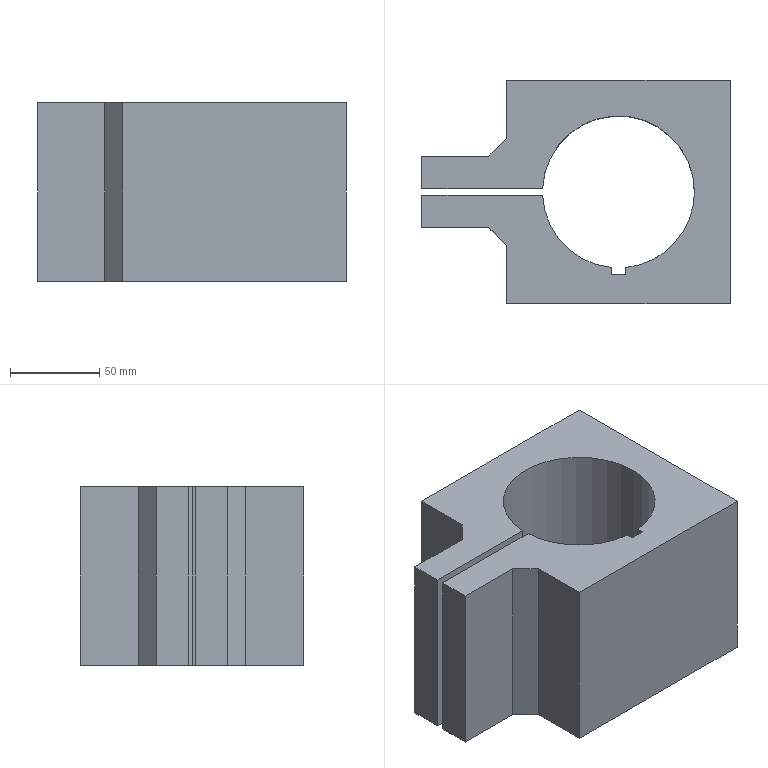Part | STEP file | csb-00001 | 1 solid | 21 faces | box 172.5 x 125 x 100 mm | volume 1165193 mm3 | plane 18 | cylinder 3 | commonest cylinder face diameters 85 x3
STEP:
#1=CARTESIAN_POINT('',(-42.453,2.,-100.));
#2=VERTEX_POINT('',#1);
#3=CARTESIAN_POINT('',(42.5,0.,-100.));
#4=VERTEX_POINT('',#3);
#5=CARTESIAN_POINT('',(0.,0.,-100.));
#6=DIRECTION('',(0.,0.,-1.));
#7=DIRECTION('',(1.,0.,0.));
#8=AXIS2_PLACEMENT_3D('',#5,#6,#7);
#9=CIRCLE('',#8,42.5);
#10=EDGE_CURVE('',#2,#4,#9,.T.);
#11=ORIENTED_EDGE('',*,*,#10,.T.);
#12=CARTESIAN_POINT('',(42.5,0.,0.));
#13=VERTEX_POINT('',#12);
#14=CARTESIAN_POINT('',(42.5,0.,-100.));
#15=DIRECTION('',(0.,0.,1.));
#16=VECTOR('',#15,1000.);
#17=LINE('',#14,#16);
#18=EDGE_CURVE('',#4,#13,#17,.T.);
#19=ORIENTED_EDGE('',*,*,#18,.T.);
#20=CARTESIAN_POINT('',(-42.453,2.,0.));
#21=VERTEX_POINT('',#20);
#22=CARTESIAN_POINT('',(0.,0.,0.));
#23=DIRECTION('',(0.,0.,-1.));
#24=DIRECTION('',(1.,0.,0.));
#25=AXIS2_PLACEMENT_3D('',#22,#23,#24);
#26=CIRCLE('',#25,42.5);
#27=EDGE_CURVE('',#21,#13,#26,.T.);
#28=ORIENTED_EDGE('',*,*,#27,.F.);
#29=CARTESIAN_POINT('',(-42.453,2.,-100.));
#30=DIRECTION('',(0.,0.,1.));
#31=VECTOR('',#30,1000.);
#32=LINE('',#29,#31);
#33=EDGE_CURVE('',#2,#21,#32,.T.);
#34=ORIENTED_EDGE('',*,*,#33,.F.);
#35=EDGE_LOOP('',(#11,#19,#28,#34));
#36=FACE_OUTER_BOUND('',#35,.T.);
#37=CARTESIAN_POINT('',(0.,0.,-100.));
#38=DIRECTION('',(0.,0.,1.));
#39=DIRECTION('',(1.,0.,0.));
#40=AXIS2_PLACEMENT_3D('',#37,#38,#39);
#41=CYLINDRICAL_SURFACE('',#40,42.5);
#42=ADVANCED_FACE('',(#36),#41,.F.);
#43=CARTESIAN_POINT('',(62.5,-62.5,0.));
#44=VERTEX_POINT('',#43);
#45=CARTESIAN_POINT('',(62.5,62.5,0.));
#46=VERTEX_POINT('',#45);
#47=CARTESIAN_POINT('',(62.5,-62.5,0.));
#48=DIRECTION('',(0.,1.,0.));
#49=VECTOR('',#48,1000.);
#50=LINE('',#47,#49);
#51=EDGE_CURVE('',#44,#46,#50,.T.);
#52=ORIENTED_EDGE('',*,*,#51,.F.);
#53=CARTESIAN_POINT('',(62.5,-62.5,-100.));
#54=VERTEX_POINT('',#53);
#55=CARTESIAN_POINT('',(62.5,-62.5,-100.));
#56=DIRECTION('',(0.,0.,1.));
#57=VECTOR('',#56,1000.);
#58=LINE('',#55,#57);
#59=EDGE_CURVE('',#54,#44,#58,.T.);
#60=ORIENTED_EDGE('',*,*,#59,.F.);
#61=CARTESIAN_POINT('',(62.5,62.5,-100.));
#62=VERTEX_POINT('',#61);
#63=CARTESIAN_POINT('',(62.5,-62.5,-100.));
#64=DIRECTION('',(0.,1.,0.));
#65=VECTOR('',#64,1000.);
#66=LINE('',#63,#65);
#67=EDGE_CURVE('',#54,#62,#66,.T.);
#68=ORIENTED_EDGE('',*,*,#67,.T.);
#69=CARTESIAN_POINT('',(62.5,62.5,-100.));
#70=DIRECTION('',(0.,0.,1.));
#71=VECTOR('',#70,1000.);
#72=LINE('',#69,#71);
#73=EDGE_CURVE('',#62,#46,#72,.T.);
#74=ORIENTED_EDGE('',*,*,#73,.T.);
#75=EDGE_LOOP('',(#52,#60,#68,#74));
#76=FACE_OUTER_BOUND('',#75,.T.);
#77=CARTESIAN_POINT('',(62.5,-62.5,-100.));
#78=DIRECTION('',(1.,0.,0.));
#79=DIRECTION('',(0.,0.,-1.));
#80=AXIS2_PLACEMENT_3D('',#77,#78,#79);
#81=PLANE('',#80);
#82=ADVANCED_FACE('',(#76),#81,.T.);
#83=CARTESIAN_POINT('',(-62.5,-62.5,0.));
#84=VERTEX_POINT('',#83);
#85=CARTESIAN_POINT('',(-62.5,-62.5,0.));
#86=DIRECTION('',(1.,0.,0.));
#87=VECTOR('',#86,1000.);
#88=LINE('',#85,#87);
#89=EDGE_CURVE('',#84,#44,#88,.T.);
#90=ORIENTED_EDGE('',*,*,#89,.F.);
#91=CARTESIAN_POINT('',(-62.5,-62.5,-100.));
#92=VERTEX_POINT('',#91);
#93=CARTESIAN_POINT('',(-62.5,-62.5,-100.));
#94=DIRECTION('',(0.,0.,1.));
#95=VECTOR('',#94,1000.);
#96=LINE('',#93,#95);
#97=EDGE_CURVE('',#92,#84,#96,.T.);
#98=ORIENTED_EDGE('',*,*,#97,.F.);
#99=CARTESIAN_POINT('',(-62.5,-62.5,-100.));
#100=DIRECTION('',(1.,0.,0.));
#101=VECTOR('',#100,1000.);
#102=LINE('',#99,#101);
#103=EDGE_CURVE('',#92,#54,#102,.T.);
#104=ORIENTED_EDGE('',*,*,#103,.T.);
#105=ORIENTED_EDGE('',*,*,#59,.T.);
#106=EDGE_LOOP('',(#90,#98,#104,#105));
#107=FACE_OUTER_BOUND('',#106,.T.);
#108=CARTESIAN_POINT('',(-62.5,-62.5,-100.));
#109=DIRECTION('',(0.,-1.,0.));
#110=DIRECTION('',(0.,0.,-1.));
#111=AXIS2_PLACEMENT_3D('',#108,#109,#110);
#112=PLANE('',#111);
#113=ADVANCED_FACE('',(#107),#112,.T.);
#114=CARTESIAN_POINT('',(-62.5,-30.,0.));
#115=VERTEX_POINT('',#114);
#116=CARTESIAN_POINT('',(-62.5,-62.5,0.));
#117=DIRECTION('',(0.,-1.,0.));
#118=VECTOR('',#117,1000.);
#119=LINE('',#116,#118);
#120=EDGE_CURVE('',#115,#84,#119,.T.);
#121=ORIENTED_EDGE('',*,*,#120,.F.);
#122=CARTESIAN_POINT('',(-62.5,-30.,-100.));
#123=VERTEX_POINT('',#122);
#124=CARTESIAN_POINT('',(-62.5,-30.,-100.));
#125=DIRECTION('',(0.,0.,1.));
#126=VECTOR('',#125,1000.);
#127=LINE('',#124,#126);
#128=EDGE_CURVE('',#123,#115,#127,.T.);
#129=ORIENTED_EDGE('',*,*,#128,.F.);
#130=CARTESIAN_POINT('',(-62.5,-62.5,-100.));
#131=DIRECTION('',(0.,-1.,0.));
#132=VECTOR('',#131,1000.);
#133=LINE('',#130,#132);
#134=EDGE_CURVE('',#123,#92,#133,.T.);
#135=ORIENTED_EDGE('',*,*,#134,.T.);
#136=ORIENTED_EDGE('',*,*,#97,.T.);
#137=EDGE_LOOP('',(#121,#129,#135,#136));
#138=FACE_OUTER_BOUND('',#137,.T.);
#139=CARTESIAN_POINT('',(-62.5,-62.5,-100.));
#140=DIRECTION('',(-1.,0.,0.));
#141=DIRECTION('',(0.,0.,1.));
#142=AXIS2_PLACEMENT_3D('',#139,#140,#141);
#143=PLANE('',#142);
#144=ADVANCED_FACE('',(#138),#143,.T.);
#145=CARTESIAN_POINT('',(-72.5,-20.,0.));
#146=VERTEX_POINT('',#145);
#147=CARTESIAN_POINT('',(-72.5,-20.,0.));
#148=DIRECTION('',(0.7071,-0.7071,0.));
#149=VECTOR('',#148,1000.);
#150=LINE('',#147,#149);
#151=EDGE_CURVE('',#146,#115,#150,.T.);
#152=ORIENTED_EDGE('',*,*,#151,.F.);
#153=CARTESIAN_POINT('',(-72.5,-20.,-100.));
#154=VERTEX_POINT('',#153);
#155=CARTESIAN_POINT('',(-72.5,-20.,-100.));
#156=DIRECTION('',(0.,0.,1.));
#157=VECTOR('',#156,1000.);
#158=LINE('',#155,#157);
#159=EDGE_CURVE('',#154,#146,#158,.T.);
#160=ORIENTED_EDGE('',*,*,#159,.F.);
#161=CARTESIAN_POINT('',(-72.5,-20.,-100.));
#162=DIRECTION('',(0.7071,-0.7071,0.));
#163=VECTOR('',#162,1000.);
#164=LINE('',#161,#163);
#165=EDGE_CURVE('',#154,#123,#164,.T.);
#166=ORIENTED_EDGE('',*,*,#165,.T.);
#167=ORIENTED_EDGE('',*,*,#128,.T.);
#168=EDGE_LOOP('',(#152,#160,#166,#167));
#169=FACE_OUTER_BOUND('',#168,.T.);
#170=CARTESIAN_POINT('',(-72.5,-20.,-100.));
#171=DIRECTION('',(-0.7071,-0.7071,0.));
#172=DIRECTION('',(0.7071,-0.7071,0.));
#173=AXIS2_PLACEMENT_3D('',#170,#171,#172);
#174=PLANE('',#173);
#175=ADVANCED_FACE('',(#169),#174,.T.);
#176=CARTESIAN_POINT('',(-110.,-20.,0.));
#177=VERTEX_POINT('',#176);
#178=CARTESIAN_POINT('',(-110.,-20.,0.));
#179=DIRECTION('',(1.,0.,0.));
#180=VECTOR('',#179,1000.);
#181=LINE('',#178,#180);
#182=EDGE_CURVE('',#177,#146,#181,.T.);
#183=ORIENTED_EDGE('',*,*,#182,.F.);
#184=CARTESIAN_POINT('',(-110.,-20.,-100.));
#185=VERTEX_POINT('',#184);
#186=CARTESIAN_POINT('',(-110.,-20.,-100.));
#187=DIRECTION('',(0.,0.,1.));
#188=VECTOR('',#187,1000.);
#189=LINE('',#186,#188);
#190=EDGE_CURVE('',#185,#177,#189,.T.);
#191=ORIENTED_EDGE('',*,*,#190,.F.);
#192=CARTESIAN_POINT('',(-110.,-20.,-100.));
#193=DIRECTION('',(1.,0.,0.));
#194=VECTOR('',#193,1000.);
#195=LINE('',#192,#194);
#196=EDGE_CURVE('',#185,#154,#195,.T.);
#197=ORIENTED_EDGE('',*,*,#196,.T.);
#198=ORIENTED_EDGE('',*,*,#159,.T.);
#199=EDGE_LOOP('',(#183,#191,#197,#198));
#200=FACE_OUTER_BOUND('',#199,.T.);
#201=CARTESIAN_POINT('',(-110.,-20.,-100.));
#202=DIRECTION('',(0.,-1.,0.));
#203=DIRECTION('',(1.,0.,0.));
#204=AXIS2_PLACEMENT_3D('',#201,#202,#203);
#205=PLANE('',#204);
#206=ADVANCED_FACE('',(#200),#205,.T.);
#207=CARTESIAN_POINT('',(-110.,-2.,0.));
#208=VERTEX_POINT('',#207);
#209=CARTESIAN_POINT('',(-110.,-20.,0.));
#210=DIRECTION('',(0.,-1.,0.));
#211=VECTOR('',#210,1000.);
#212=LINE('',#209,#211);
#213=EDGE_CURVE('',#208,#177,#212,.T.);
#214=ORIENTED_EDGE('',*,*,#213,.F.);
#215=CARTESIAN_POINT('',(-110.,-2.,-100.));
#216=VERTEX_POINT('',#215);
#217=CARTESIAN_POINT('',(-110.,-2.,-100.));
#218=DIRECTION('',(0.,0.,1.));
#219=VECTOR('',#218,1000.);
#220=LINE('',#217,#219);
#221=EDGE_CURVE('',#216,#208,#220,.T.);
#222=ORIENTED_EDGE('',*,*,#221,.F.);
#223=CARTESIAN_POINT('',(-110.,-20.,-100.));
#224=DIRECTION('',(0.,-1.,0.));
#225=VECTOR('',#224,1000.);
#226=LINE('',#223,#225);
#227=EDGE_CURVE('',#216,#185,#226,.T.);
#228=ORIENTED_EDGE('',*,*,#227,.T.);
#229=ORIENTED_EDGE('',*,*,#190,.T.);
#230=EDGE_LOOP('',(#214,#222,#228,#229));
#231=FACE_OUTER_BOUND('',#230,.T.);
#232=CARTESIAN_POINT('',(-110.,-20.,-100.));
#233=DIRECTION('',(-1.,0.,0.));
#234=DIRECTION('',(0.,-1.,0.));
#235=AXIS2_PLACEMENT_3D('',#232,#233,#234);
#236=PLANE('',#235);
#237=ADVANCED_FACE('',(#231),#236,.T.);
#238=CARTESIAN_POINT('',(-42.453,-2.,0.));
#239=VERTEX_POINT('',#238);
#240=CARTESIAN_POINT('',(-110.,-2.,0.));
#241=DIRECTION('',(-1.,0.,0.));
#242=VECTOR('',#241,1000.);
#243=LINE('',#240,#242);
#244=EDGE_CURVE('',#239,#208,#243,.T.);
#245=ORIENTED_EDGE('',*,*,#244,.F.);
#246=CARTESIAN_POINT('',(-42.453,-2.,-100.));
#247=VERTEX_POINT('',#246);
#248=CARTESIAN_POINT('',(-42.453,-2.,-100.));
#249=DIRECTION('',(0.,0.,1.));
#250=VECTOR('',#249,1000.);
#251=LINE('',#248,#250);
#252=EDGE_CURVE('',#247,#239,#251,.T.);
#253=ORIENTED_EDGE('',*,*,#252,.F.);
#254=CARTESIAN_POINT('',(-110.,-2.,-100.));
#255=DIRECTION('',(-1.,0.,0.));
#256=VECTOR('',#255,1000.);
#257=LINE('',#254,#256);
#258=EDGE_CURVE('',#247,#216,#257,.T.);
#259=ORIENTED_EDGE('',*,*,#258,.T.);
#260=ORIENTED_EDGE('',*,*,#221,.T.);
#261=EDGE_LOOP('',(#245,#253,#259,#260));
#262=FACE_OUTER_BOUND('',#261,.T.);
#263=CARTESIAN_POINT('',(-110.,-2.,-100.));
#264=DIRECTION('',(0.,1.,0.));
#265=DIRECTION('',(0.,0.,1.));
#266=AXIS2_PLACEMENT_3D('',#263,#264,#265);
#267=PLANE('',#266);
#268=ADVANCED_FACE('',(#262),#267,.T.);
#269=CARTESIAN_POINT('',(-4.,-42.311,0.));
#270=VERTEX_POINT('',#269);
#271=CARTESIAN_POINT('',(0.,0.,0.));
#272=DIRECTION('',(0.,0.,-1.));
#273=DIRECTION('',(1.,0.,0.));
#274=AXIS2_PLACEMENT_3D('',#271,#272,#273);
#275=CIRCLE('',#274,42.5);
#276=EDGE_CURVE('',#270,#239,#275,.T.);
#277=ORIENTED_EDGE('',*,*,#276,.F.);
#278=CARTESIAN_POINT('',(-4.,-42.311,-100.));
#279=VERTEX_POINT('',#278);
#280=CARTESIAN_POINT('',(-4.,-42.311,-100.));
#281=DIRECTION('',(0.,0.,1.));
#282=VECTOR('',#281,1000.);
#283=LINE('',#280,#282);
#284=EDGE_CURVE('',#279,#270,#283,.T.);
#285=ORIENTED_EDGE('',*,*,#284,.F.);
#286=CARTESIAN_POINT('',(0.,0.,-100.));
#287=DIRECTION('',(0.,0.,-1.));
#288=DIRECTION('',(1.,0.,0.));
#289=AXIS2_PLACEMENT_3D('',#286,#287,#288);
#290=CIRCLE('',#289,42.5);
#291=EDGE_CURVE('',#279,#247,#290,.T.);
#292=ORIENTED_EDGE('',*,*,#291,.T.);
#293=ORIENTED_EDGE('',*,*,#252,.T.);
#294=EDGE_LOOP('',(#277,#285,#292,#293));
#295=FACE_OUTER_BOUND('',#294,.T.);
#296=CARTESIAN_POINT('',(0.,0.,-100.));
#297=DIRECTION('',(0.,0.,1.));
#298=DIRECTION('',(1.,0.,0.));
#299=AXIS2_PLACEMENT_3D('',#296,#297,#298);
#300=CYLINDRICAL_SURFACE('',#299,42.5);
#301=ADVANCED_FACE('',(#295),#300,.F.);
#302=CARTESIAN_POINT('',(-4.,-46.,0.));
#303=VERTEX_POINT('',#302);
#304=CARTESIAN_POINT('',(-4.,-46.,0.));
#305=DIRECTION('',(0.,1.,0.));
#306=VECTOR('',#305,1000.);
#307=LINE('',#304,#306);
#308=EDGE_CURVE('',#303,#270,#307,.T.);
#309=ORIENTED_EDGE('',*,*,#308,.F.);
#310=CARTESIAN_POINT('',(-4.,-46.,-100.));
#311=VERTEX_POINT('',#310);
#312=CARTESIAN_POINT('',(-4.,-46.,-100.));
#313=DIRECTION('',(0.,0.,1.));
#314=VECTOR('',#313,1000.);
#315=LINE('',#312,#314);
#316=EDGE_CURVE('',#311,#303,#315,.T.);
#317=ORIENTED_EDGE('',*,*,#316,.F.);
#318=CARTESIAN_POINT('',(-4.,-46.,-100.));
#319=DIRECTION('',(0.,1.,0.));
#320=VECTOR('',#319,1000.);
#321=LINE('',#318,#320);
#322=EDGE_CURVE('',#311,#279,#321,.T.);
#323=ORIENTED_EDGE('',*,*,#322,.T.);
#324=ORIENTED_EDGE('',*,*,#284,.T.);
#325=EDGE_LOOP('',(#309,#317,#323,#324));
#326=FACE_OUTER_BOUND('',#325,.T.);
#327=CARTESIAN_POINT('',(-4.,-46.,-100.));
#328=DIRECTION('',(1.,0.,0.));
#329=DIRECTION('',(0.,1.,0.));
#330=AXIS2_PLACEMENT_3D('',#327,#328,#329);
#331=PLANE('',#330);
#332=ADVANCED_FACE('',(#326),#331,.T.);
#333=CARTESIAN_POINT('',(4.,-46.,0.));
#334=VERTEX_POINT('',#333);
#335=CARTESIAN_POINT('',(-4.,-46.,0.));
#336=DIRECTION('',(-1.,0.,0.));
#337=VECTOR('',#336,1000.);
#338=LINE('',#335,#337);
#339=EDGE_CURVE('',#334,#303,#338,.T.);
#340=ORIENTED_EDGE('',*,*,#339,.F.);
#341=CARTESIAN_POINT('',(4.,-46.,-100.));
#342=VERTEX_POINT('',#341);
#343=CARTESIAN_POINT('',(4.,-46.,-100.));
#344=DIRECTION('',(0.,0.,1.));
#345=VECTOR('',#344,1000.);
#346=LINE('',#343,#345);
#347=EDGE_CURVE('',#342,#334,#346,.T.);
#348=ORIENTED_EDGE('',*,*,#347,.F.);
#349=CARTESIAN_POINT('',(-4.,-46.,-100.));
#350=DIRECTION('',(-1.,0.,0.));
#351=VECTOR('',#350,1000.);
#352=LINE('',#349,#351);
#353=EDGE_CURVE('',#342,#311,#352,.T.);
#354=ORIENTED_EDGE('',*,*,#353,.T.);
#355=ORIENTED_EDGE('',*,*,#316,.T.);
#356=EDGE_LOOP('',(#340,#348,#354,#355));
#357=FACE_OUTER_BOUND('',#356,.T.);
#358=CARTESIAN_POINT('',(-4.,-46.,-100.));
#359=DIRECTION('',(0.,1.,0.));
#360=DIRECTION('',(-1.,0.,0.));
#361=AXIS2_PLACEMENT_3D('',#358,#359,#360);
#362=PLANE('',#361);
#363=ADVANCED_FACE('',(#357),#362,.T.);
#364=CARTESIAN_POINT('',(4.,-42.311,0.));
#365=VERTEX_POINT('',#364);
#366=CARTESIAN_POINT('',(4.,-46.,0.));
#367=DIRECTION('',(0.,-1.,0.));
#368=VECTOR('',#367,1000.);
#369=LINE('',#366,#368);
#370=EDGE_CURVE('',#365,#334,#369,.T.);
#371=ORIENTED_EDGE('',*,*,#370,.F.);
#372=CARTESIAN_POINT('',(4.,-42.311,-100.));
#373=VERTEX_POINT('',#372);
#374=CARTESIAN_POINT('',(4.,-42.311,-100.));
#375=DIRECTION('',(0.,0.,1.));
#376=VECTOR('',#375,1000.);
#377=LINE('',#374,#376);
#378=EDGE_CURVE('',#373,#365,#377,.T.);
#379=ORIENTED_EDGE('',*,*,#378,.F.);
#380=CARTESIAN_POINT('',(4.,-46.,-100.));
#381=DIRECTION('',(0.,-1.,0.));
#382=VECTOR('',#381,1000.);
#383=LINE('',#380,#382);
#384=EDGE_CURVE('',#373,#342,#383,.T.);
#385=ORIENTED_EDGE('',*,*,#384,.T.);
#386=ORIENTED_EDGE('',*,*,#347,.T.);
#387=EDGE_LOOP('',(#371,#379,#385,#386));
#388=FACE_OUTER_BOUND('',#387,.T.);
#389=CARTESIAN_POINT('',(4.,-46.,-100.));
#390=DIRECTION('',(-1.,0.,0.));
#391=DIRECTION('',(0.,0.,1.));
#392=AXIS2_PLACEMENT_3D('',#389,#390,#391);
#393=PLANE('',#392);
#394=ADVANCED_FACE('',(#388),#393,.T.);
#395=ORIENTED_EDGE('',*,*,#18,.F.);
#396=CARTESIAN_POINT('',(0.,0.,-100.));
#397=DIRECTION('',(0.,0.,-1.));
#398=DIRECTION('',(1.,0.,0.));
#399=AXIS2_PLACEMENT_3D('',#396,#397,#398);
#400=CIRCLE('',#399,42.5);
#401=EDGE_CURVE('',#4,#373,#400,.T.);
#402=ORIENTED_EDGE('',*,*,#401,.T.);
#403=ORIENTED_EDGE('',*,*,#378,.T.);
#404=CARTESIAN_POINT('',(0.,0.,0.));
#405=DIRECTION('',(0.,0.,-1.));
#406=DIRECTION('',(1.,0.,0.));
#407=AXIS2_PLACEMENT_3D('',#404,#405,#406);
#408=CIRCLE('',#407,42.5);
#409=EDGE_CURVE('',#13,#365,#408,.T.);
#410=ORIENTED_EDGE('',*,*,#409,.F.);
#411=EDGE_LOOP('',(#395,#402,#403,#410));
#412=FACE_OUTER_BOUND('',#411,.T.);
#413=CARTESIAN_POINT('',(0.,0.,-100.));
#414=DIRECTION('',(0.,0.,1.));
#415=DIRECTION('',(1.,0.,0.));
#416=AXIS2_PLACEMENT_3D('',#413,#414,#415);
#417=CYLINDRICAL_SURFACE('',#416,42.5);
#418=ADVANCED_FACE('',(#412),#417,.F.);
#419=CARTESIAN_POINT('',(-110.,2.,0.));
#420=VERTEX_POINT('',#419);
#421=CARTESIAN_POINT('',(-110.,2.,0.));
#422=DIRECTION('',(1.,0.,0.));
#423=VECTOR('',#422,1000.);
#424=LINE('',#421,#423);
#425=EDGE_CURVE('',#420,#21,#424,.T.);
#426=ORIENTED_EDGE('',*,*,#425,.F.);
#427=CARTESIAN_POINT('',(-110.,2.,-100.));
#428=VERTEX_POINT('',#427);
#429=CARTESIAN_POINT('',(-110.,2.,-100.));
#430=DIRECTION('',(0.,0.,1.));
#431=VECTOR('',#430,1000.);
#432=LINE('',#429,#431);
#433=EDGE_CURVE('',#428,#420,#432,.T.);
#434=ORIENTED_EDGE('',*,*,#433,.F.);
#435=CARTESIAN_POINT('',(-110.,2.,-100.));
#436=DIRECTION('',(1.,0.,0.));
#437=VECTOR('',#436,1000.);
#438=LINE('',#435,#437);
#439=EDGE_CURVE('',#428,#2,#438,.T.);
#440=ORIENTED_EDGE('',*,*,#439,.T.);
#441=ORIENTED_EDGE('',*,*,#33,.T.);
#442=EDGE_LOOP('',(#426,#434,#440,#441));
#443=FACE_OUTER_BOUND('',#442,.T.);
#444=CARTESIAN_POINT('',(-110.,2.,-100.));
#445=DIRECTION('',(0.,-1.,0.));
#446=DIRECTION('',(0.,0.,-1.));
#447=AXIS2_PLACEMENT_3D('',#444,#445,#446);
#448=PLANE('',#447);
#449=ADVANCED_FACE('',(#443),#448,.T.);
#450=CARTESIAN_POINT('',(-110.,20.,0.));
#451=VERTEX_POINT('',#450);
#452=CARTESIAN_POINT('',(-110.,2.,0.));
#453=DIRECTION('',(0.,-1.,0.));
#454=VECTOR('',#453,1000.);
#455=LINE('',#452,#454);
#456=EDGE_CURVE('',#451,#420,#455,.T.);
#457=ORIENTED_EDGE('',*,*,#456,.F.);
#458=CARTESIAN_POINT('',(-110.,20.,-100.));
#459=VERTEX_POINT('',#458);
#460=CARTESIAN_POINT('',(-110.,20.,-100.));
#461=DIRECTION('',(0.,0.,1.));
#462=VECTOR('',#461,1000.);
#463=LINE('',#460,#462);
#464=EDGE_CURVE('',#459,#451,#463,.T.);
#465=ORIENTED_EDGE('',*,*,#464,.F.);
#466=CARTESIAN_POINT('',(-110.,2.,-100.));
#467=DIRECTION('',(0.,-1.,0.));
#468=VECTOR('',#467,1000.);
#469=LINE('',#466,#468);
#470=EDGE_CURVE('',#459,#428,#469,.T.);
#471=ORIENTED_EDGE('',*,*,#470,.T.);
#472=ORIENTED_EDGE('',*,*,#433,.T.);
#473=EDGE_LOOP('',(#457,#465,#471,#472));
#474=FACE_OUTER_BOUND('',#473,.T.);
#475=CARTESIAN_POINT('',(-110.,2.,-100.));
#476=DIRECTION('',(-1.,0.,0.));
#477=DIRECTION('',(0.,-1.,0.));
#478=AXIS2_PLACEMENT_3D('',#475,#476,#477);
#479=PLANE('',#478);
#480=ADVANCED_FACE('',(#474),#479,.T.);
#481=CARTESIAN_POINT('',(-72.5,20.,0.));
#482=VERTEX_POINT('',#481);
#483=CARTESIAN_POINT('',(-110.,20.,0.));
#484=DIRECTION('',(-1.,0.,0.));
#485=VECTOR('',#484,1000.);
#486=LINE('',#483,#485);
#487=EDGE_CURVE('',#482,#451,#486,.T.);
#488=ORIENTED_EDGE('',*,*,#487,.F.);
#489=CARTESIAN_POINT('',(-72.5,20.,-100.));
#490=VERTEX_POINT('',#489);
#491=CARTESIAN_POINT('',(-72.5,20.,-100.));
#492=DIRECTION('',(0.,0.,1.));
#493=VECTOR('',#492,1000.);
#494=LINE('',#491,#493);
#495=EDGE_CURVE('',#490,#482,#494,.T.);
#496=ORIENTED_EDGE('',*,*,#495,.F.);
#497=CARTESIAN_POINT('',(-110.,20.,-100.));
#498=DIRECTION('',(-1.,0.,0.));
#499=VECTOR('',#498,1000.);
#500=LINE('',#497,#499);
#501=EDGE_CURVE('',#490,#459,#500,.T.);
#502=ORIENTED_EDGE('',*,*,#501,.T.);
#503=ORIENTED_EDGE('',*,*,#464,.T.);
#504=EDGE_LOOP('',(#488,#496,#502,#503));
#505=FACE_OUTER_BOUND('',#504,.T.);
#506=CARTESIAN_POINT('',(-110.,20.,-100.));
#507=DIRECTION('',(0.,1.,0.));
#508=DIRECTION('',(-1.,0.,0.));
#509=AXIS2_PLACEMENT_3D('',#506,#507,#508);
#510=PLANE('',#509);
#511=ADVANCED_FACE('',(#505),#510,.T.);
#512=CARTESIAN_POINT('',(-62.5,30.,0.));
#513=VERTEX_POINT('',#512);
#514=CARTESIAN_POINT('',(-72.5,20.,0.));
#515=DIRECTION('',(-0.7071,-0.7071,0.));
#516=VECTOR('',#515,1000.);
#517=LINE('',#514,#516);
#518=EDGE_CURVE('',#513,#482,#517,.T.);
#519=ORIENTED_EDGE('',*,*,#518,.F.);
#520=CARTESIAN_POINT('',(-62.5,30.,-100.));
#521=VERTEX_POINT('',#520);
#522=CARTESIAN_POINT('',(-62.5,30.,-100.));
#523=DIRECTION('',(0.,0.,1.));
#524=VECTOR('',#523,1000.);
#525=LINE('',#522,#524);
#526=EDGE_CURVE('',#521,#513,#525,.T.);
#527=ORIENTED_EDGE('',*,*,#526,.F.);
#528=CARTESIAN_POINT('',(-72.5,20.,-100.));
#529=DIRECTION('',(-0.7071,-0.7071,0.));
#530=VECTOR('',#529,1000.);
#531=LINE('',#528,#530);
#532=EDGE_CURVE('',#521,#490,#531,.T.);
#533=ORIENTED_EDGE('',*,*,#532,.T.);
#534=ORIENTED_EDGE('',*,*,#495,.T.);
#535=EDGE_LOOP('',(#519,#527,#533,#534));
#536=FACE_OUTER_BOUND('',#535,.T.);
#537=CARTESIAN_POINT('',(-72.5,20.,-100.));
#538=DIRECTION('',(-0.7071,0.7071,0.));
#539=DIRECTION('',(-0.7071,-0.7071,0.));
#540=AXIS2_PLACEMENT_3D('',#537,#538,#539);
#541=PLANE('',#540);
#542=ADVANCED_FACE('',(#536),#541,.T.);
#543=CARTESIAN_POINT('',(-62.5,62.5,0.));
#544=VERTEX_POINT('',#543);
#545=CARTESIAN_POINT('',(-62.5,30.,0.));
#546=DIRECTION('',(0.,-1.,0.));
#547=VECTOR('',#546,1000.);
#548=LINE('',#545,#547);
#549=EDGE_CURVE('',#544,#513,#548,.T.);
#550=ORIENTED_EDGE('',*,*,#549,.F.);
#551=CARTESIAN_POINT('',(-62.5,62.5,-100.));
#552=VERTEX_POINT('',#551);
#553=CARTESIAN_POINT('',(-62.5,62.5,-100.));
#554=DIRECTION('',(0.,0.,1.));
#555=VECTOR('',#554,1000.);
#556=LINE('',#553,#555);
#557=EDGE_CURVE('',#552,#544,#556,.T.);
#558=ORIENTED_EDGE('',*,*,#557,.F.);
#559=CARTESIAN_POINT('',(-62.5,30.,-100.));
#560=DIRECTION('',(0.,-1.,0.));
#561=VECTOR('',#560,1000.);
#562=LINE('',#559,#561);
#563=EDGE_CURVE('',#552,#521,#562,.T.);
#564=ORIENTED_EDGE('',*,*,#563,.T.);
#565=ORIENTED_EDGE('',*,*,#526,.T.);
#566=EDGE_LOOP('',(#550,#558,#564,#565));
#567=FACE_OUTER_BOUND('',#566,.T.);
#568=CARTESIAN_POINT('',(-62.5,30.,-100.));
#569=DIRECTION('',(-1.,0.,0.));
#570=DIRECTION('',(0.,0.,1.));
#571=AXIS2_PLACEMENT_3D('',#568,#569,#570);
#572=PLANE('',#571);
#573=ADVANCED_FACE('',(#567),#572,.T.);
#574=CARTESIAN_POINT('',(-62.5,62.5,0.));
#575=DIRECTION('',(-1.,0.,0.));
#576=VECTOR('',#575,1000.);
#577=LINE('',#574,#576);
#578=EDGE_CURVE('',#46,#544,#577,.T.);
#579=ORIENTED_EDGE('',*,*,#578,.F.);
#580=ORIENTED_EDGE('',*,*,#73,.F.);
#581=CARTESIAN_POINT('',(-62.5,62.5,-100.));
#582=DIRECTION('',(-1.,0.,0.));
#583=VECTOR('',#582,1000.);
#584=LINE('',#581,#583);
#585=EDGE_CURVE('',#62,#552,#584,.T.);
#586=ORIENTED_EDGE('',*,*,#585,.T.);
#587=ORIENTED_EDGE('',*,*,#557,.T.);
#588=EDGE_LOOP('',(#579,#580,#586,#587));
#589=FACE_OUTER_BOUND('',#588,.T.);
#590=CARTESIAN_POINT('',(-62.5,62.5,-100.));
#591=DIRECTION('',(0.,1.,0.));
#592=DIRECTION('',(0.,0.,1.));
#593=AXIS2_PLACEMENT_3D('',#590,#591,#592);
#594=PLANE('',#593);
#595=ADVANCED_FACE('',(#589),#594,.T.);
#596=ORIENTED_EDGE('',*,*,#67,.F.);
#597=ORIENTED_EDGE('',*,*,#103,.F.);
#598=ORIENTED_EDGE('',*,*,#134,.F.);
#599=ORIENTED_EDGE('',*,*,#165,.F.);
#600=ORIENTED_EDGE('',*,*,#196,.F.);
#601=ORIENTED_EDGE('',*,*,#227,.F.);
#602=ORIENTED_EDGE('',*,*,#258,.F.);
#603=ORIENTED_EDGE('',*,*,#291,.F.);
#604=ORIENTED_EDGE('',*,*,#322,.F.);
#605=ORIENTED_EDGE('',*,*,#353,.F.);
#606=ORIENTED_EDGE('',*,*,#384,.F.);
#607=ORIENTED_EDGE('',*,*,#401,.F.);
#608=ORIENTED_EDGE('',*,*,#10,.F.);
#609=ORIENTED_EDGE('',*,*,#439,.F.);
#610=ORIENTED_EDGE('',*,*,#470,.F.);
#611=ORIENTED_EDGE('',*,*,#501,.F.);
#612=ORIENTED_EDGE('',*,*,#532,.F.);
#613=ORIENTED_EDGE('',*,*,#563,.F.);
#614=ORIENTED_EDGE('',*,*,#585,.F.);
#615=EDGE_LOOP('',(#596,#597,#598,#599,#600,#601,#602,#603,#604,#605,#606,#607,#608,#609,#610,#611,#612,#613,#614));
#616=FACE_OUTER_BOUND('',#615,.T.);
#617=CARTESIAN_POINT('',(0.,0.,-100.));
#618=DIRECTION('',(0.,0.,1.));
#619=DIRECTION('',(1.,0.,0.));
#620=AXIS2_PLACEMENT_3D('',#617,#618,#619);
#621=PLANE('',#620);
#622=ADVANCED_FACE('',(#616),#621,.F.);
#623=ORIENTED_EDGE('',*,*,#51,.T.);
#624=ORIENTED_EDGE('',*,*,#578,.T.);
#625=ORIENTED_EDGE('',*,*,#549,.T.);
#626=ORIENTED_EDGE('',*,*,#518,.T.);
#627=ORIENTED_EDGE('',*,*,#487,.T.);
#628=ORIENTED_EDGE('',*,*,#456,.T.);
#629=ORIENTED_EDGE('',*,*,#425,.T.);
#630=ORIENTED_EDGE('',*,*,#27,.T.);
#631=ORIENTED_EDGE('',*,*,#409,.T.);
#632=ORIENTED_EDGE('',*,*,#370,.T.);
#633=ORIENTED_EDGE('',*,*,#339,.T.);
#634=ORIENTED_EDGE('',*,*,#308,.T.);
#635=ORIENTED_EDGE('',*,*,#276,.T.);
#636=ORIENTED_EDGE('',*,*,#244,.T.);
#637=ORIENTED_EDGE('',*,*,#213,.T.);
#638=ORIENTED_EDGE('',*,*,#182,.T.);
#639=ORIENTED_EDGE('',*,*,#151,.T.);
#640=ORIENTED_EDGE('',*,*,#120,.T.);
#641=ORIENTED_EDGE('',*,*,#89,.T.);
#642=EDGE_LOOP('',(#623,#624,#625,#626,#627,#628,#629,#630,#631,#632,#633,#634,#635,#636,#637,#638,#639,#640,#641));
#643=FACE_OUTER_BOUND('',#642,.T.);
#644=CARTESIAN_POINT('',(0.,0.,0.));
#645=DIRECTION('',(0.,0.,1.));
#646=DIRECTION('',(1.,0.,0.));
#647=AXIS2_PLACEMENT_3D('',#644,#645,#646);
#648=PLANE('',#647);
#649=ADVANCED_FACE('',(#643),#648,.T.);
#650=CLOSED_SHELL('',(#42,#82,#113,#144,#175,#206,#237,#268,#301,#332,#363,#394,#418,#449,#480,#511,#542,#573,#595,#622,#649));
#651=MANIFOLD_SOLID_BREP('',#650);
#652=CARTESIAN_POINT('',(0.,0.,0.));
#653=DIRECTION('',(0.,0.,1.));
#654=DIRECTION('',(1.,0.,0.));
#655=AXIS2_PLACEMENT_3D('',#652,#653,#654);
#656=(LENGTH_UNIT()NAMED_UNIT(*)SI_UNIT(.MILLI.,.METRE.));
#657=UNCERTAINTY_MEASURE_WITH_UNIT(LENGTH_MEASURE(0.00001),#656,'','');
#658=(NAMED_UNIT(*)PLANE_ANGLE_UNIT()SI_UNIT($,.RADIAN.));
#659=(NAMED_UNIT(*)SI_UNIT($,.STERADIAN.)SOLID_ANGLE_UNIT());
#660=(GEOMETRIC_REPRESENTATION_CONTEXT(3)GLOBAL_UNCERTAINTY_ASSIGNED_CONTEXT((#657))GLOBAL_UNIT_ASSIGNED_CONTEXT((#656,#658,#659))REPRESENTATION_CONTEXT('',''));
#661=ADVANCED_BREP_SHAPE_REPRESENTATION('',(#651,#655),#660);